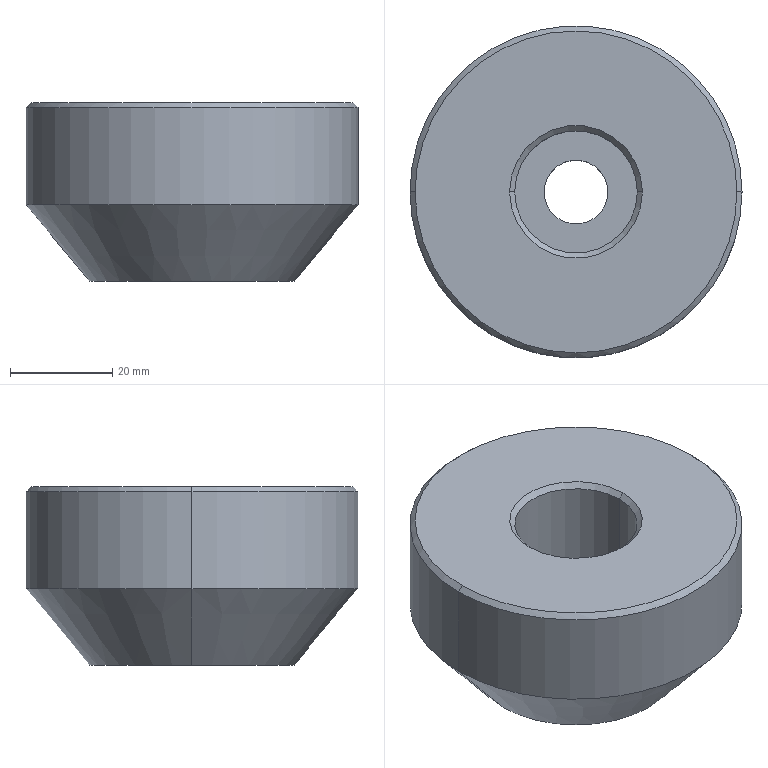Part | STEP file | Foot pad shim | 1 solid | 15 faces | box 65 x 65 x 35 mm | volume 88423 mm3 | cylinder 6 | cone 6 | plane 3 | commonest cylinder face diameters 12.5 x2 24 x2 65 x2
STEP:
#1=CARTESIAN_POINT('',(-6.25,0.,-35.));
#2=VERTEX_POINT('',#1);
#3=CARTESIAN_POINT('',(6.25,0.,-35.));
#4=VERTEX_POINT('',#3);
#5=CARTESIAN_POINT('',(0.,0.,-35.));
#6=DIRECTION('',(0.,0.,1.));
#7=DIRECTION('',(1.,0.,0.));
#8=AXIS2_PLACEMENT_3D('',#5,#6,#7);
#9=CIRCLE('',#8,6.25);
#10=EDGE_CURVE('',#2,#4,#9,.T.);
#11=ORIENTED_EDGE('',*,*,#10,.F.);
#12=CARTESIAN_POINT('',(-6.25,0.,-20.));
#13=VERTEX_POINT('',#12);
#14=CARTESIAN_POINT('',(-6.25,0.,-35.));
#15=DIRECTION('',(0.,0.,1.));
#16=VECTOR('',#15,1000.);
#17=LINE('',#14,#16);
#18=EDGE_CURVE('',#2,#13,#17,.T.);
#19=ORIENTED_EDGE('',*,*,#18,.T.);
#20=CARTESIAN_POINT('',(6.25,0.,-20.));
#21=VERTEX_POINT('',#20);
#22=CARTESIAN_POINT('',(0.,0.,-20.));
#23=DIRECTION('',(0.,0.,1.));
#24=DIRECTION('',(1.,0.,0.));
#25=AXIS2_PLACEMENT_3D('',#22,#23,#24);
#26=CIRCLE('',#25,6.25);
#27=EDGE_CURVE('',#13,#21,#26,.T.);
#28=ORIENTED_EDGE('',*,*,#27,.T.);
#29=CARTESIAN_POINT('',(6.25,0.,-35.));
#30=DIRECTION('',(0.,0.,1.));
#31=VECTOR('',#30,1000.);
#32=LINE('',#29,#31);
#33=EDGE_CURVE('',#4,#21,#32,.T.);
#34=ORIENTED_EDGE('',*,*,#33,.F.);
#35=EDGE_LOOP('',(#11,#19,#28,#34));
#36=FACE_OUTER_BOUND('',#35,.T.);
#37=CARTESIAN_POINT('',(0.,0.,-35.));
#38=DIRECTION('',(0.,0.,1.));
#39=DIRECTION('',(1.,0.,0.));
#40=AXIS2_PLACEMENT_3D('',#37,#38,#39);
#41=CYLINDRICAL_SURFACE('',#40,6.25);
#42=ADVANCED_FACE('',(#36),#41,.F.);
#43=CARTESIAN_POINT('',(-12.,0.,-1.));
#44=VERTEX_POINT('',#43);
#45=CARTESIAN_POINT('',(12.,0.,-1.));
#46=VERTEX_POINT('',#45);
#47=CARTESIAN_POINT('',(0.,0.,-1.));
#48=DIRECTION('',(0.,0.,1.));
#49=DIRECTION('',(-1.,0.,0.));
#50=AXIS2_PLACEMENT_3D('',#47,#48,#49);
#51=CIRCLE('',#50,12.);
#52=EDGE_CURVE('',#44,#46,#51,.T.);
#53=ORIENTED_EDGE('',*,*,#52,.F.);
#54=CARTESIAN_POINT('',(-13.,0.,0.));
#55=VERTEX_POINT('',#54);
#56=CARTESIAN_POINT('',(-12.,0.,-1.));
#57=DIRECTION('',(-0.7071,0.,0.7071));
#58=VECTOR('',#57,1000.);
#59=LINE('',#56,#58);
#60=EDGE_CURVE('',#44,#55,#59,.T.);
#61=ORIENTED_EDGE('',*,*,#60,.T.);
#62=CARTESIAN_POINT('',(13.,0.,0.));
#63=VERTEX_POINT('',#62);
#64=CARTESIAN_POINT('',(0.,0.,0.));
#65=DIRECTION('',(0.,0.,-1.));
#66=DIRECTION('',(-1.,0.,0.));
#67=AXIS2_PLACEMENT_3D('',#64,#65,#66);
#68=CIRCLE('',#67,13.);
#69=EDGE_CURVE('',#63,#55,#68,.T.);
#70=ORIENTED_EDGE('',*,*,#69,.F.);
#71=CARTESIAN_POINT('',(12.,0.,-1.));
#72=DIRECTION('',(0.7071,0.,0.7071));
#73=VECTOR('',#72,1000.);
#74=LINE('',#71,#73);
#75=EDGE_CURVE('',#46,#63,#74,.T.);
#76=ORIENTED_EDGE('',*,*,#75,.F.);
#77=EDGE_LOOP('',(#53,#61,#70,#76));
#78=FACE_OUTER_BOUND('',#77,.T.);
#79=CARTESIAN_POINT('',(0.,0.,-1.));
#80=DIRECTION('',(0.,0.,1.));
#81=DIRECTION('',(1.,0.,0.));
#82=AXIS2_PLACEMENT_3D('',#79,#80,#81);
#83=CONICAL_SURFACE('',#82,12.,0.7854);
#84=ADVANCED_FACE('',(#78),#83,.F.);
#85=CARTESIAN_POINT('',(-12.,0.,-20.));
#86=VERTEX_POINT('',#85);
#87=CARTESIAN_POINT('',(12.,0.,-20.));
#88=VERTEX_POINT('',#87);
#89=CARTESIAN_POINT('',(0.,0.,-20.));
#90=DIRECTION('',(0.,0.,1.));
#91=DIRECTION('',(1.,0.,0.));
#92=AXIS2_PLACEMENT_3D('',#89,#90,#91);
#93=CIRCLE('',#92,12.);
#94=EDGE_CURVE('',#86,#88,#93,.T.);
#95=ORIENTED_EDGE('',*,*,#94,.F.);
#96=CARTESIAN_POINT('',(-12.,0.,-20.));
#97=DIRECTION('',(0.,0.,1.));
#98=VECTOR('',#97,1000.);
#99=LINE('',#96,#98);
#100=EDGE_CURVE('',#86,#44,#99,.T.);
#101=ORIENTED_EDGE('',*,*,#100,.T.);
#102=ORIENTED_EDGE('',*,*,#52,.T.);
#103=CARTESIAN_POINT('',(12.,0.,-20.));
#104=DIRECTION('',(0.,0.,1.));
#105=VECTOR('',#104,1000.);
#106=LINE('',#103,#105);
#107=EDGE_CURVE('',#88,#46,#106,.T.);
#108=ORIENTED_EDGE('',*,*,#107,.F.);
#109=EDGE_LOOP('',(#95,#101,#102,#108));
#110=FACE_OUTER_BOUND('',#109,.T.);
#111=CARTESIAN_POINT('',(0.,0.,-20.));
#112=DIRECTION('',(0.,0.,1.));
#113=DIRECTION('',(1.,0.,0.));
#114=AXIS2_PLACEMENT_3D('',#111,#112,#113);
#115=CYLINDRICAL_SURFACE('',#114,12.);
#116=ADVANCED_FACE('',(#110),#115,.F.);
#117=CARTESIAN_POINT('',(31.5,0.,0.));
#118=VERTEX_POINT('',#117);
#119=CARTESIAN_POINT('',(-31.5,0.,0.));
#120=VERTEX_POINT('',#119);
#121=CARTESIAN_POINT('',(0.,0.,0.));
#122=DIRECTION('',(0.,0.,1.));
#123=DIRECTION('',(-1.,0.,0.));
#124=AXIS2_PLACEMENT_3D('',#121,#122,#123);
#125=CIRCLE('',#124,31.5);
#126=EDGE_CURVE('',#118,#120,#125,.T.);
#127=ORIENTED_EDGE('',*,*,#126,.F.);
#128=CARTESIAN_POINT('',(32.5,0.,-1.));
#129=VERTEX_POINT('',#128);
#130=CARTESIAN_POINT('',(32.5,0.,-1.));
#131=DIRECTION('',(0.7071,0.,-0.7071));
#132=VECTOR('',#131,1000.);
#133=LINE('',#130,#132);
#134=EDGE_CURVE('',#118,#129,#133,.T.);
#135=ORIENTED_EDGE('',*,*,#134,.T.);
#136=CARTESIAN_POINT('',(-32.5,0.,-1.));
#137=VERTEX_POINT('',#136);
#138=CARTESIAN_POINT('',(0.,0.,-1.));
#139=DIRECTION('',(0.,0.,-1.));
#140=DIRECTION('',(-1.,0.,0.));
#141=AXIS2_PLACEMENT_3D('',#138,#139,#140);
#142=CIRCLE('',#141,32.5);
#143=EDGE_CURVE('',#137,#129,#142,.T.);
#144=ORIENTED_EDGE('',*,*,#143,.F.);
#145=CARTESIAN_POINT('',(-32.5,0.,-1.));
#146=DIRECTION('',(-0.7071,0.,-0.7071));
#147=VECTOR('',#146,1000.);
#148=LINE('',#145,#147);
#149=EDGE_CURVE('',#120,#137,#148,.T.);
#150=ORIENTED_EDGE('',*,*,#149,.F.);
#151=EDGE_LOOP('',(#127,#135,#144,#150));
#152=FACE_OUTER_BOUND('',#151,.T.);
#153=CARTESIAN_POINT('',(0.,0.,-1.));
#154=DIRECTION('',(0.,0.,-1.));
#155=DIRECTION('',(-1.,0.,0.));
#156=AXIS2_PLACEMENT_3D('',#153,#154,#155);
#157=CONICAL_SURFACE('',#156,32.5,0.7854);
#158=ADVANCED_FACE('',(#152),#157,.T.);
#159=CARTESIAN_POINT('',(-20.,0.,-35.));
#160=VERTEX_POINT('',#159);
#161=CARTESIAN_POINT('',(20.,0.,-35.));
#162=VERTEX_POINT('',#161);
#163=CARTESIAN_POINT('',(0.,0.,-35.));
#164=DIRECTION('',(0.,0.,-1.));
#165=DIRECTION('',(-1.,0.,0.));
#166=AXIS2_PLACEMENT_3D('',#163,#164,#165);
#167=CIRCLE('',#166,20.);
#168=EDGE_CURVE('',#160,#162,#167,.T.);
#169=ORIENTED_EDGE('',*,*,#168,.F.);
#170=CARTESIAN_POINT('',(-32.5,0.,-20.));
#171=VERTEX_POINT('',#170);
#172=CARTESIAN_POINT('',(-32.5,0.,-20.));
#173=DIRECTION('',(-0.6402,0.,0.7682));
#174=VECTOR('',#173,1000.);
#175=LINE('',#172,#174);
#176=EDGE_CURVE('',#160,#171,#175,.T.);
#177=ORIENTED_EDGE('',*,*,#176,.T.);
#178=CARTESIAN_POINT('',(32.5,0.,-20.));
#179=VERTEX_POINT('',#178);
#180=CARTESIAN_POINT('',(0.,0.,-20.));
#181=DIRECTION('',(0.,0.,-1.));
#182=DIRECTION('',(-1.,0.,0.));
#183=AXIS2_PLACEMENT_3D('',#180,#181,#182);
#184=CIRCLE('',#183,32.5);
#185=EDGE_CURVE('',#171,#179,#184,.T.);
#186=ORIENTED_EDGE('',*,*,#185,.T.);
#187=CARTESIAN_POINT('',(32.5,0.,-20.));
#188=DIRECTION('',(0.6402,0.,0.7682));
#189=VECTOR('',#188,1000.);
#190=LINE('',#187,#189);
#191=EDGE_CURVE('',#162,#179,#190,.T.);
#192=ORIENTED_EDGE('',*,*,#191,.F.);
#193=EDGE_LOOP('',(#169,#177,#186,#192));
#194=FACE_OUTER_BOUND('',#193,.T.);
#195=CARTESIAN_POINT('',(0.,0.,-20.));
#196=DIRECTION('',(0.,0.,1.));
#197=DIRECTION('',(1.,0.,0.));
#198=AXIS2_PLACEMENT_3D('',#195,#196,#197);
#199=CONICAL_SURFACE('',#198,32.5,0.6947);
#200=ADVANCED_FACE('',(#194),#199,.T.);
#201=ORIENTED_EDGE('',*,*,#143,.T.);
#202=CARTESIAN_POINT('',(32.5,0.,-64.696));
#203=DIRECTION('',(0.,0.,-1.));
#204=VECTOR('',#203,1000.);
#205=LINE('',#202,#204);
#206=EDGE_CURVE('',#129,#179,#205,.T.);
#207=ORIENTED_EDGE('',*,*,#206,.T.);
#208=ORIENTED_EDGE('',*,*,#185,.F.);
#209=CARTESIAN_POINT('',(-32.5,0.,-64.696));
#210=DIRECTION('',(0.,0.,-1.));
#211=VECTOR('',#210,1000.);
#212=LINE('',#209,#211);
#213=EDGE_CURVE('',#137,#171,#212,.T.);
#214=ORIENTED_EDGE('',*,*,#213,.F.);
#215=EDGE_LOOP('',(#201,#207,#208,#214));
#216=FACE_OUTER_BOUND('',#215,.T.);
#217=CARTESIAN_POINT('',(0.,0.,-64.696));
#218=DIRECTION('',(0.,0.,-1.));
#219=DIRECTION('',(-1.,0.,0.));
#220=AXIS2_PLACEMENT_3D('',#217,#218,#219);
#221=CYLINDRICAL_SURFACE('',#220,32.5);
#222=ADVANCED_FACE('',(#216),#221,.T.);
#223=ORIENTED_EDGE('',*,*,#69,.T.);
#224=CARTESIAN_POINT('',(0.,0.,0.));
#225=DIRECTION('',(0.,0.,-1.));
#226=DIRECTION('',(-1.,0.,0.));
#227=AXIS2_PLACEMENT_3D('',#224,#225,#226);
#228=CIRCLE('',#227,13.);
#229=EDGE_CURVE('',#55,#63,#228,.T.);
#230=ORIENTED_EDGE('',*,*,#229,.T.);
#231=EDGE_LOOP('',(#223,#230));
#232=FACE_BOUND('',#231,.T.);
#233=CARTESIAN_POINT('',(0.,0.,0.));
#234=DIRECTION('',(0.,0.,1.));
#235=DIRECTION('',(-1.,0.,0.));
#236=AXIS2_PLACEMENT_3D('',#233,#234,#235);
#237=CIRCLE('',#236,31.5);
#238=EDGE_CURVE('',#120,#118,#237,.T.);
#239=ORIENTED_EDGE('',*,*,#238,.T.);
#240=ORIENTED_EDGE('',*,*,#126,.T.);
#241=EDGE_LOOP('',(#239,#240));
#242=FACE_OUTER_BOUND('',#241,.T.);
#243=CARTESIAN_POINT('',(0.,0.,0.));
#244=DIRECTION('',(0.,0.,-1.));
#245=DIRECTION('',(-1.,0.,0.));
#246=AXIS2_PLACEMENT_3D('',#243,#244,#245);
#247=PLANE('',#246);
#248=ADVANCED_FACE('',(#232,#242),#247,.F.);
#249=ORIENTED_EDGE('',*,*,#206,.F.);
#250=CARTESIAN_POINT('',(0.,0.,-1.));
#251=DIRECTION('',(0.,0.,-1.));
#252=DIRECTION('',(-1.,0.,0.));
#253=AXIS2_PLACEMENT_3D('',#250,#251,#252);
#254=CIRCLE('',#253,32.5);
#255=EDGE_CURVE('',#129,#137,#254,.T.);
#256=ORIENTED_EDGE('',*,*,#255,.T.);
#257=ORIENTED_EDGE('',*,*,#213,.T.);
#258=CARTESIAN_POINT('',(0.,0.,-20.));
#259=DIRECTION('',(0.,0.,-1.));
#260=DIRECTION('',(-1.,0.,0.));
#261=AXIS2_PLACEMENT_3D('',#258,#259,#260);
#262=CIRCLE('',#261,32.5);
#263=EDGE_CURVE('',#179,#171,#262,.T.);
#264=ORIENTED_EDGE('',*,*,#263,.F.);
#265=EDGE_LOOP('',(#249,#256,#257,#264));
#266=FACE_OUTER_BOUND('',#265,.T.);
#267=CARTESIAN_POINT('',(0.,0.,-64.696));
#268=DIRECTION('',(0.,0.,-1.));
#269=DIRECTION('',(-1.,0.,0.));
#270=AXIS2_PLACEMENT_3D('',#267,#268,#269);
#271=CYLINDRICAL_SURFACE('',#270,32.5);
#272=ADVANCED_FACE('',(#266),#271,.T.);
#273=ORIENTED_EDGE('',*,*,#176,.F.);
#274=CARTESIAN_POINT('',(0.,0.,-35.));
#275=DIRECTION('',(0.,0.,-1.));
#276=DIRECTION('',(-1.,0.,0.));
#277=AXIS2_PLACEMENT_3D('',#274,#275,#276);
#278=CIRCLE('',#277,20.);
#279=EDGE_CURVE('',#162,#160,#278,.T.);
#280=ORIENTED_EDGE('',*,*,#279,.F.);
#281=ORIENTED_EDGE('',*,*,#191,.T.);
#282=ORIENTED_EDGE('',*,*,#263,.T.);
#283=EDGE_LOOP('',(#273,#280,#281,#282));
#284=FACE_OUTER_BOUND('',#283,.T.);
#285=CARTESIAN_POINT('',(0.,0.,-20.));
#286=DIRECTION('',(0.,0.,1.));
#287=DIRECTION('',(1.,0.,0.));
#288=AXIS2_PLACEMENT_3D('',#285,#286,#287);
#289=CONICAL_SURFACE('',#288,32.5,0.6947);
#290=ADVANCED_FACE('',(#284),#289,.T.);
#291=CARTESIAN_POINT('',(0.,0.,-35.));
#292=DIRECTION('',(0.,0.,1.));
#293=DIRECTION('',(1.,0.,0.));
#294=AXIS2_PLACEMENT_3D('',#291,#292,#293);
#295=CIRCLE('',#294,6.25);
#296=EDGE_CURVE('',#4,#2,#295,.T.);
#297=ORIENTED_EDGE('',*,*,#296,.T.);
#298=ORIENTED_EDGE('',*,*,#10,.T.);
#299=EDGE_LOOP('',(#297,#298));
#300=FACE_BOUND('',#299,.T.);
#301=ORIENTED_EDGE('',*,*,#279,.T.);
#302=ORIENTED_EDGE('',*,*,#168,.T.);
#303=EDGE_LOOP('',(#301,#302));
#304=FACE_OUTER_BOUND('',#303,.T.);
#305=CARTESIAN_POINT('',(20.,0.,-35.));
#306=DIRECTION('',(0.,0.,1.));
#307=DIRECTION('',(1.,0.,0.));
#308=AXIS2_PLACEMENT_3D('',#305,#306,#307);
#309=PLANE('',#308);
#310=ADVANCED_FACE('',(#300,#304),#309,.F.);
#311=ORIENTED_EDGE('',*,*,#134,.F.);
#312=ORIENTED_EDGE('',*,*,#238,.F.);
#313=ORIENTED_EDGE('',*,*,#149,.T.);
#314=ORIENTED_EDGE('',*,*,#255,.F.);
#315=EDGE_LOOP('',(#311,#312,#313,#314));
#316=FACE_OUTER_BOUND('',#315,.T.);
#317=CARTESIAN_POINT('',(0.,0.,-1.));
#318=DIRECTION('',(0.,0.,-1.));
#319=DIRECTION('',(-1.,0.,0.));
#320=AXIS2_PLACEMENT_3D('',#317,#318,#319);
#321=CONICAL_SURFACE('',#320,32.5,0.7854);
#322=ADVANCED_FACE('',(#316),#321,.T.);
#323=ORIENTED_EDGE('',*,*,#100,.F.);
#324=CARTESIAN_POINT('',(0.,0.,-20.));
#325=DIRECTION('',(0.,0.,1.));
#326=DIRECTION('',(1.,0.,0.));
#327=AXIS2_PLACEMENT_3D('',#324,#325,#326);
#328=CIRCLE('',#327,12.);
#329=EDGE_CURVE('',#88,#86,#328,.T.);
#330=ORIENTED_EDGE('',*,*,#329,.F.);
#331=ORIENTED_EDGE('',*,*,#107,.T.);
#332=CARTESIAN_POINT('',(0.,0.,-1.));
#333=DIRECTION('',(0.,0.,1.));
#334=DIRECTION('',(-1.,0.,0.));
#335=AXIS2_PLACEMENT_3D('',#332,#333,#334);
#336=CIRCLE('',#335,12.);
#337=EDGE_CURVE('',#46,#44,#336,.T.);
#338=ORIENTED_EDGE('',*,*,#337,.T.);
#339=EDGE_LOOP('',(#323,#330,#331,#338));
#340=FACE_OUTER_BOUND('',#339,.T.);
#341=CARTESIAN_POINT('',(0.,0.,-20.));
#342=DIRECTION('',(0.,0.,1.));
#343=DIRECTION('',(1.,0.,0.));
#344=AXIS2_PLACEMENT_3D('',#341,#342,#343);
#345=CYLINDRICAL_SURFACE('',#344,12.);
#346=ADVANCED_FACE('',(#340),#345,.F.);
#347=CARTESIAN_POINT('',(0.,0.,-20.));
#348=DIRECTION('',(0.,0.,1.));
#349=DIRECTION('',(1.,0.,0.));
#350=AXIS2_PLACEMENT_3D('',#347,#348,#349);
#351=CIRCLE('',#350,6.25);
#352=EDGE_CURVE('',#21,#13,#351,.T.);
#353=ORIENTED_EDGE('',*,*,#352,.F.);
#354=ORIENTED_EDGE('',*,*,#27,.F.);
#355=EDGE_LOOP('',(#353,#354));
#356=FACE_BOUND('',#355,.T.);
#357=ORIENTED_EDGE('',*,*,#329,.T.);
#358=ORIENTED_EDGE('',*,*,#94,.T.);
#359=EDGE_LOOP('',(#357,#358));
#360=FACE_OUTER_BOUND('',#359,.T.);
#361=CARTESIAN_POINT('',(0.,0.,-20.));
#362=DIRECTION('',(0.,0.,1.));
#363=DIRECTION('',(1.,0.,0.));
#364=AXIS2_PLACEMENT_3D('',#361,#362,#363);
#365=PLANE('',#364);
#366=ADVANCED_FACE('',(#356,#360),#365,.T.);
#367=ORIENTED_EDGE('',*,*,#60,.F.);
#368=ORIENTED_EDGE('',*,*,#337,.F.);
#369=ORIENTED_EDGE('',*,*,#75,.T.);
#370=ORIENTED_EDGE('',*,*,#229,.F.);
#371=EDGE_LOOP('',(#367,#368,#369,#370));
#372=FACE_OUTER_BOUND('',#371,.T.);
#373=CARTESIAN_POINT('',(0.,0.,-1.));
#374=DIRECTION('',(0.,0.,1.));
#375=DIRECTION('',(1.,0.,0.));
#376=AXIS2_PLACEMENT_3D('',#373,#374,#375);
#377=CONICAL_SURFACE('',#376,12.,0.7854);
#378=ADVANCED_FACE('',(#372),#377,.F.);
#379=ORIENTED_EDGE('',*,*,#18,.F.);
#380=ORIENTED_EDGE('',*,*,#296,.F.);
#381=ORIENTED_EDGE('',*,*,#33,.T.);
#382=ORIENTED_EDGE('',*,*,#352,.T.);
#383=EDGE_LOOP('',(#379,#380,#381,#382));
#384=FACE_OUTER_BOUND('',#383,.T.);
#385=CARTESIAN_POINT('',(0.,0.,-35.));
#386=DIRECTION('',(0.,0.,1.));
#387=DIRECTION('',(1.,0.,0.));
#388=AXIS2_PLACEMENT_3D('',#385,#386,#387);
#389=CYLINDRICAL_SURFACE('',#388,6.25);
#390=ADVANCED_FACE('',(#384),#389,.F.);
#391=CLOSED_SHELL('',(#42,#84,#116,#158,#200,#222,#248,#272,#290,#310,#322,#346,#366,#378,#390));
#392=MANIFOLD_SOLID_BREP('',#391);
#393=CARTESIAN_POINT('',(0.,0.,0.));
#394=DIRECTION('',(0.,0.,1.));
#395=DIRECTION('',(1.,0.,0.));
#396=AXIS2_PLACEMENT_3D('',#393,#394,#395);
#397=(LENGTH_UNIT()NAMED_UNIT(*)SI_UNIT(.MILLI.,.METRE.));
#398=UNCERTAINTY_MEASURE_WITH_UNIT(LENGTH_MEASURE(0.00001),#397,'','');
#399=(NAMED_UNIT(*)PLANE_ANGLE_UNIT()SI_UNIT($,.RADIAN.));
#400=(NAMED_UNIT(*)SI_UNIT($,.STERADIAN.)SOLID_ANGLE_UNIT());
#401=(GEOMETRIC_REPRESENTATION_CONTEXT(3)GLOBAL_UNCERTAINTY_ASSIGNED_CONTEXT((#398))GLOBAL_UNIT_ASSIGNED_CONTEXT((#397,#399,#400))REPRESENTATION_CONTEXT('',''));
#402=ADVANCED_BREP_SHAPE_REPRESENTATION('',(#392,#396),#401);